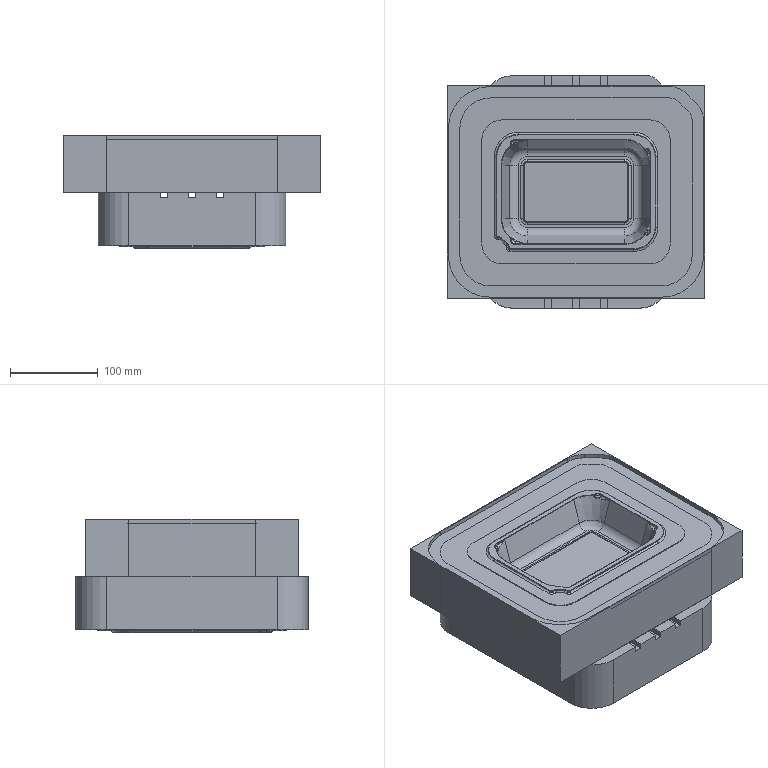NC program | NX | posted with a generic post | part box 293.342 x 265.342 x 129.5 mm
Lines 5002 to 6050 of 68427:
(B2 , TOOL : D8)
N10002 M6
N10004 G53
N10006 G17 G0 G90 X-89.051 Y-62.969 S7000 M3 M8
N10008 G43 Z215.5 H0
N10010 Z64.916
N10012 G94 G1 Z63.916 F4500.
N10014 X-86.104 Y-60.021
N10016 G3 X-86.104 Y-57.758 R1.6
N10018 G1 X-88.036 Y-55.826
N10020 G3 X-88.557 Y-55.61 R0.738
N10022 G1 X-89.227
N10024 G2 X-91.115 Y-55.286 R5.85
N10026 G3 X-93.151 Y-56.272 R1.6
N10028 G1 X-94.414 Y-59.905
N10030 Z64.916
N10032 G0 Z68.5
N10034 X-88.832 Y-63.392
N10036 Z64.582
N10038 G1 Z63.582
N10040 X-85.884 Y-60.444
N10042 G3 X-85.884 Y-58.182 R1.6
N10044 G1 X-88.119 Y-55.947
N10046 G3 X-88.585 Y-55.755 R0.659
N10048 G1 X-89.29
N10050 G2 X-91.54 Y-55.316 R5.876
N10052 G3 X-93.628 Y-56.189 R1.6
N10054 G1 X-95.087 Y-59.749
N10056 Z64.582
N10058 G0 Z68.5
N10060 X-85.268 Y-69.101
N10062 Z64.916
N10064 G1 Z63.916
N10066 X-81.645 Y-67.81
N10068 G3 X-80.676 Y-65.765 R1.6
N10070 G2 X-81.012 Y-63.966 R5.823
N10072 G1 X-81.021 Y-63.576
N10074 Y-63.147
N10076 G3 X-81.237 Y-62.625 R0.738
N10078 G1 X-83.165 Y-60.697
N10080 G3 X-85.428 Y-60.697 R1.6
N10082 G1 X-88.376 Y-63.645
N10084 Z64.916
N10086 G0 Z68.5
N10088 X-85.235 Y-69.546
N10090 Z64.582
N10092 G1 Z63.582
N10094 X-81.657 Y-68.134
N10096 G3 X-80.755 Y-66.059 R1.6
N10098 G2 X-81.165 Y-63.88 R5.875
N10100 G1 Y-63.173
N10102 G3 X-81.358 Y-62.708 R0.657
N10104 G1 X-83.586 Y-60.48
N10106 G3 X-85.849 Y-60.48 R1.6
N10108 G1 X-88.797 Y-63.428
N10110 Z64.582
N10112 G0 Z67.25
N10114 X-3.207 Y-76.775
N10116 Z64.248
N10118 G1 Z63.248
N10120 Y-71.505
N10122 G3 X-4.807 Y-69.905 R1.6
N10124 G1 X-75.383
N10126 G2 X-79.615 Y-68.143 R5.962
N10128 X-81.293 Y-63.949 R5.976
N10130 G1 Y-63.204
N10132 G3 X-81.468 Y-62.778 R0.602
N10134 G1 X-88.16 Y-56.086
N10136 G3 X-88.615 Y-55.882 R0.651
N10138 G1 X-89.43
N10140 G2 X-95.315 Y-49.996 R5.886
N10142 G1 Y40.358
N10144 G2 X-65.769 Y69.905 R29.546
N10146 G1 X65.769
N10148 G2 X95.315 Y40.358 R29.546
N10150 G1 Y-40.358
N10152 G2 X65.769 Y-69.905 R29.546
N10154 G1 X-4.807
N10156 G3 X-6.407 Y-71.505 R1.6
N10158 G1 Y-76.775
N10160 Z64.248
N10162 G0 Z66.582
N10164 X-3.207 Y-76.932
N10166 Z63.914
N10168 G1 Z62.914
N10170 Y-71.689
N10172 G3 X-4.807 Y-70.089 R1.6
N10174 G1 X-75.337
N10176 G2 X-81.476 Y-63.949 R6.037
N10178 G1 Y-63.242
N10180 G3 X-81.598 Y-62.908 R0.465
N10182 G1 X-88.314 Y-56.192
N10184 X-88.615 Y-56.066
N10186 X-89.359
N10188 G2 X-95.499 Y-49.926 R6.031
N10190 G1 Y40.358
N10192 G2 X-65.769 Y70.089 R29.73
N10194 G1 X65.769
N10196 G2 X95.499 Y40.358 R29.73
N10198 G1 Y-40.358
N10200 G2 X65.769 Y-70.089 R29.73
N10202 G1 X-4.807
N10204 G3 X-6.407 Y-71.689 R1.6
N10206 G1 Y-76.932
N10208 Z63.914
N10210 G0 Z67.25
N10212 X-89.345 Y-63.704
N10214 Z63.58
N10216 G1 Z62.58
N10218 X-86.397 Y-60.756
N10220 G3 X-86.397 Y-58.494 R1.6
N10222 G1 X-88.553 Y-56.338
N10224 X-89.359
N10226 G2 X-91.454 Y-56.019 R6.301
N10228 G3 X-93.476 Y-57.034 R1.6
N10230 G1 X-94.693 Y-60.705
N10232 Z63.58
N10234 G0 Z65.914
N10236 X-89.681 Y-63.963
N10238 Z63.246
N10240 G1 Z62.246
N10242 X-86.733 Y-61.015
N10244 G3 X-86.733 Y-58.753 R1.6
N10246 G1 X-88.727 Y-56.758
N10248 X-89.359
N10250 G2 X-91.462 Y-56.462 R6.706
N10252 G3 X-93.462 Y-57.52 R1.6
N10254 G1 X-94.606 Y-61.233
N10256 Z63.246
N10258 G0 Z65.58
N10260 X-90.266 Y-65.371
N10262 Z62.912
N10264 G1 Z61.912
N10266 X-87.026 Y-62.131
N10268 G3 X-87.026 Y-59.868 R1.6
N10270 G1 X-89.14 Y-57.754
N10272 X-89.359
N10274 X-89.736 Y-57.835
N10276 G2 X-91.734 Y-57.498 R8.299
N10278 G3 X-93.725 Y-58.574 R1.6
N10280 G1 X-94.849 Y-62.347
N10282 Z62.912
N10284 G0 Z65.914
N10286 X-86.139 Y-69.234
N10288 Z63.58
N10290 G1 Z62.58
N10292 X-82.463 Y-68.034
N10294 G3 X-81.438 Y-66.016 R1.6
N10296 G2 X-81.749 Y-63.949 R6.302
N10298 G1 Y-63.201
N10300 X-81.886 Y-63.005
N10302 X-83.898 Y-60.993
N10304 G3 X-86.161 Y-60.993 R1.6
N10306 G1 X-89.109 Y-63.941
N10308 Z63.58
N10310 G0 Z65.914
N10312 X-86.659 Y-69.16
N10314 Z63.246
N10316 G1 Z62.246
N10318 X-82.943 Y-68.027
N10320 G3 X-81.879 Y-66.031 R1.6
N10322 G2 X-82.169 Y-63.949 R6.707
N10324 G1 Y-63.316
N10326 X-84.157 Y-61.328
N10328 G3 X-86.42 Y-61.328 R1.6
N10330 G1 X-89.368 Y-64.276
N10332 Z63.246
N10334 G0 Z65.58
N10336 X-87.614 Y-69.717
N10338 Z62.912
N10340 G1 Z61.912
N10342 X-83.89 Y-68.513
N10344 G3 X-82.86 Y-66.499 R1.6
N10346 G2 X-83.136 Y-65.35 R7.681
N10348 G1 X-83.227 Y-64.658
N10350 X-83.165 Y-63.949
N10352 Y-63.729
N10354 X-85.305 Y-61.589
N10356 G3 X-87.568 Y-61.589 R1.6
N10358 G1 X-90.808 Y-64.828
N10360 Z62.912
N10362 G0 Z68.5
N10364 X-66.93 Y-46.786
N10366 Z64.916
N10368 G1 Z63.916
N10370 X-70.311 Y-48.522
N10372 G3 X-71.004 Y-50.676 R1.6
N10374 G2 X-70.442 Y-52.922 R5.1
N10376 G1 Y-54.729
N10378 G3 X-69.808 Y-55.362 R0.633
N10380 G1 X-65.313
N10382 G3 X-63.713 Y-53.762 R1.6
N10384 G1 Y-49.593
N10386 Z64.916
N10388 G0 Z68.5
N10390 X-67.282 Y-46.097
N10392 Z64.582
N10394 G1 Z63.582
N10396 X-70.524 Y-48.081
N10398 G3 X-71.054 Y-50.28 R1.6
N10400 G2 X-70.304 Y-52.9 R5.102
N10402 G1 Y-54.544
N10404 G3 X-69.617 Y-55.224 R0.637
N10406 G1 X-64.814
N10408 G3 X-63.214 Y-53.624 R1.6
N10410 G1 Y-49.455
N10412 Z64.582
N10414 G0 Z66.916
N10416 X-67.155 Y-46.069
N10418 Z64.248
N10420 G1 Z63.248
N10422 X-70.394 Y-48.045
N10424 G3 X-70.927 Y-50.244 R1.6
N10426 G2 X-70.195 Y-52.85 R5.005
N10428 G1 Y-54.428
N10430 G3 X-69.511 Y-55.116 R0.644
N10432 G1 X-64.717
N10434 G3 X-63.117 Y-53.516 R1.6
N10436 G1 Y-49.347
N10438 Z64.248
N10440 G0 Z66.582
N10442 X-67.095 Y-45.962
N10444 Z63.914
N10446 G1 Z62.914
N10448 X-70.321 Y-47.96
N10450 G3 X-70.838 Y-50.163 R1.6
N10452 G2 X-70.087 Y-52.8 R5.005
N10454 G1 Y-54.315
N10456 G3 X-69.399 Y-55.007 R0.645
N10458 G1 X-64.62
N10460 G3 X-63.02 Y-53.407 R1.6
N10462 G1 Y-49.238
N10464 Z63.914
N10466 G0 Z66.248
N10468 X-69.492 Y-43.606
N10470 Z63.58
N10472 G1 Z62.58
N10474 X-72.057 Y-46.534
N10476 G3 X-71.908 Y-48.792 R1.6
N10478 X-71.712 Y-48.962 R24.638
N10480 G2 X-69.978 Y-52.758 R4.995
N10482 G1 Y-54.08
N10484 G3 X-69.917 Y-54.513 R1.113
N10486 X-69.374 Y-54.898 R0.576
N10488 G1 X-55.815
N10490 X-55.672 Y-54.899
N10492 X-54.63
N10494 G3 X-53.03 Y-53.299 R1.6
N10496 G1 Y-49.129
N10498 Z63.58
N10500 G0 Z65.914
N10502 X-69.673 Y-42.848
N10504 Z63.246
N10506 G1 Z62.246
N10508 X-72.526 Y-45.89
N10510 G3 X-72.454 Y-48.151 R1.6
N10512 X-71.529 Y-48.976 R24.529
N10514 G2 X-69.832 Y-52.758 R4.93
N10516 G1 Y-53.896
N10518 X-69.768 Y-54.483
N10520 G3 X-69.314 Y-54.753 R0.536
N10522 G1 X-57.028
N10524 G3 X-55.672 Y-54.79 R24.529
N10526 G1 X-55.334
N10528 G3 X-53.734 Y-53.19 R1.6
N10530 G1 Y-48.984
N10532 Z63.246
N10534 G0 Z65.58
N10536 X-69.614 Y-42.69
N10538 Z62.912
N10540 G1 Z61.912
N10542 X-72.507 Y-45.754
N10544 G3 X-72.443 Y-48.015 R1.6
N10546 X-71.323 Y-49.01 R24.423
N10548 G2 X-69.625 Y-52.758 R4.854
N10550 G1 Y-54.235
N10552 G3 X-69.314 Y-54.546 R0.311
N10554 G1 X-58.27
N10556 G3 X-56.425 Y-54.673 R24.423
N10558 X-54.776 Y-53.123 R1.6
N10560 G1 X-54.645 Y-48.89
N10562 Z62.912
N10564 G0 Z65.246
N10566 X-66.724 Y-45.618
N10568 Z62.592
N10570 G1 Z61.592
N10572 X-69.8 Y-47.794
N10574 G3 X-70.182 Y-50.024 R1.6
N10576 G2 X-69.328 Y-52.711 R4.652
N10578 G1 Y-54.235
N10580 X-69.232 Y-54.248
N10582 X-64.5
N10584 G3 X-62.9 Y-52.648 R1.6
N10586 G1 Y-48.48
N10588 Z62.592
N10590 G0 Z64.912
N10592 X-66.784 Y-45.346
N10594 Z62.271
N10596 G1 Z61.271
N10598 X-69.734 Y-47.722
N10600 G3 X-69.976 Y-49.972 R1.6
N10602 G2 X-68.89 Y-52.941 R4.914
N10604 G1 Y-53.81
N10606 X-64.25
N10608 G3 X-62.65 Y-52.21 R1.6
N10610 G1 Y-48.041
N10612 Z62.271
N10614 G0 Z64.592
N10616 X-68.403 Y-43.794
N10618 Z61.951
N10620 G1 Z60.951
N10622 X-70.883 Y-46.932
N10624 G3 X-70.62 Y-49.179 R1.6
N10626 X-70.395 Y-49.354 R24.111
N10628 G2 X-68.028 Y-52.783 R6.451
N10630 G1 X-68.027 Y-52.798
N10632 X-68.013 Y-52.795
N10634 X-66.143
N10636 X-66.157 Y-52.699
N10638 X-66.066
N10640 G2 X-64.16 Y-53.051 R56.561
N10642 G3 X-64.168 Y-52.478 R2.
N10644 X-65.979 Y-51.121 R1.6
N10646 G1 X-63.674 Y-46.427
N10648 Z61.951
N10650 G0 Z68.5
N10652 X-63.691 Y49.593
N10654 Z64.916
N10656 G1 Z63.916
N10658 Y53.762
N10660 G3 X-65.291 Y55.362 R1.6
N10662 G1 X-69.794
N10664 G3 X-70.442 Y54.715 R0.648
N10666 G1 Y52.922
N10668 G2 X-71.009 Y50.666 R5.1
N10670 G3 X-70.321 Y48.51 R1.6
N10672 G1 X-66.944 Y46.767
N10674 Z64.916
N10676 G0 Z68.5
N10678 X-63.214 Y49.455
N10680 Z64.582
N10682 G1 Z63.582
N10684 Y53.624
N10686 G3 X-64.814 Y55.224 R1.6
N10688 G1 X-69.614
N10690 G3 X-70.304 Y54.544 R0.638
N10692 G1 Y52.9
N10694 G2 X-71.056 Y50.277 R5.106
N10696 G3 X-70.528 Y48.077 R1.6
N10698 G1 X-67.287 Y46.091
N10700 Z64.582
N10702 G0 Z66.916
N10704 X-63.116 Y49.347
N10706 Z64.248
N10708 G1 Z63.248
N10710 Y53.516
N10712 G3 X-64.716 Y55.116 R1.6
N10714 G1 X-69.51
N10716 G3 X-70.195 Y54.427 R0.644
N10718 G1 Y52.85
N10720 G2 X-70.933 Y50.235 R5.005
N10722 G3 X-70.405 Y48.034 R1.6
N10724 G1 X-67.169 Y46.052
N10726 Z64.248
N10728 G0 Z66.582
N10730 X-63.018 Y49.238
N10732 Z63.914
N10734 G1 Z62.914
N10736 Y53.407
N10738 G3 X-64.618 Y55.007 R1.6
N10740 G1 X-69.406
N10742 G3 X-70.087 Y54.314 R0.644
N10744 G1 Y52.8
N10746 G2 X-70.849 Y50.144 R5.005
N10748 G3 X-70.342 Y47.939 R1.6
N10750 G1 X-67.126 Y45.926
N10752 Z63.914
N10754 G0 Z66.248
N10756 X-53.149 Y49.129
N10758 Z63.58
N10760 G1 Z62.58
N10762 Y53.299
N10764 G3 X-54.749 Y54.899 R1.6
N10766 G1 X-55.672
N10768 G3 X-55.877 Y54.898 R24.638
N10770 G1 X-69.314
N10772 G3 X-69.914 Y54.541 R0.627
N10774 X-69.978 Y54.26 R0.655
N10776 G1 Y52.873
N10778 G2 X-71.712 Y48.962 R4.989
N10780 G1 X-71.801 Y48.886
N10782 G3 X-71.963 Y46.629 R1.6
N10784 G1 X-69.45 Y43.727
N10786 Z63.58
N10788 G0 Z65.914
N10790 X-53.714 Y48.984
N10792 Z63.246
N10794 G1 Z62.246
N10796 Y53.19
N10798 G3 X-55.314 Y54.79 R1.6
N10800 G1 X-55.672
N10802 G3 X-57.028 Y54.753 R24.529
N10804 G1 X-69.314
N10806 G3 X-69.77 Y54.477 R0.532
N10808 G1 X-69.832 Y53.896
N10810 Y52.758
N10812 G2 X-71.529 Y48.976 R4.93
N10814 G3 X-72.464 Y48.141 R24.529
N10816 X-72.535 Y45.879 R1.6
N10818 G1 X-69.678 Y42.837
N10820 Z63.246
N10822 G0 Z65.58
N10824 X-54.645 Y48.89
N10826 Z62.912
N10828 G1 Z61.912
N10830 X-54.776 Y53.123
N10832 G3 X-56.425 Y54.673 R1.6
N10834 X-58.27 Y54.546 R24.423
N10836 G1 X-69.314
N10838 G3 X-69.625 Y54.235 R0.311
N10840 G1 Y52.627
N10842 G2 X-71.315 Y49.017 R4.701
N10844 G3 X-72.291 Y48.158 R24.423
N10846 X-72.374 Y45.897 R1.6
N10848 G1 X-69.524 Y42.828
N10850 Z62.912
N10852 G0 Z65.246
N10854 X-62.901 Y48.48
N10856 Z62.592
N10858 G1 Z61.592
N10860 Y52.648
N10862 G3 X-64.501 Y54.248 R1.6
N10864 G1 X-69.328
N10866 Y52.792
N10868 G2 X-70.173 Y50.035 R4.642
N10870 G3 X-69.785 Y47.805 R1.6
N10872 G1 X-66.704 Y45.638
N10874 Z62.592
N10876 G0 Z64.912
N10878 X-62.623 Y48.041
N10880 Z62.271
N10882 G1 Z61.271
N10884 Y52.21
N10886 G3 X-64.223 Y53.81 R1.6
N10888 G1 X-68.89
N10890 Y52.941
N10892 G2 X-70.051 Y49.875 R4.855
N10894 G3 X-69.873 Y47.619 R1.6
N10896 G1 X-66.995 Y45.163
N10898 Z62.271
N10900 G0 Z64.592
N10902 X-63.694 Y46.406
N10904 Z61.951
N10906 G1 Z60.951
N10908 X-65.981 Y51.107
N10910 G3 X-64.17 Y52.463 R1.6
N10912 G1 X-64.164 Y52.511
N10914 G3 X-64.162 Y53.07 R2.
N10916 G1 X-64.384 Y53.021
N10918 X-64.904 Y52.902
N10920 X-65.023 Y52.844
N10922 G2 X-66.066 Y52.699 R6.755
N10924 G1 X-66.157
N10926 X-66.143 Y52.795
N10928 X-67.846
N10930 X-68.017 Y52.869
N10932 G2 X-70.395 Y49.354 R6.386
N10934 G3 X-70.626 Y49.174 R24.111
N10936 X-70.889 Y46.926 R1.6
N10938 G1 X-68.408 Y43.788
N10940 Z61.951
N10942 G0 Z64.271
N10944 X-1.6 Y-36.055
N10946 Z31.906
N10948 G1 Z30.906
N10950 Y-41.259
N10952 G3 X0. Y-42.859 R1.6
N10954 G1 X-55.672
N10956 G2 X-68.27 Y-30.261 R12.598
N10958 G1 Y30.261
N10960 G2 X-55.672 Y42.859 R12.598
N10962 G1 X55.672
N10964 G2 X68.27 Y30.261 R12.598
N10966 G1 Y-30.261
N10968 G2 X55.672 Y-42.859 R12.598
N10970 G1 X0.
N10972 G3 X1.6 Y-41.259 R1.6
N10974 G1 Y-36.055
N10976 Z31.906
N10978 G0 Z34.255
N10980 X-1.6 Y-35.567
N10982 Z31.558
N10984 G1 Z30.558
N10986 Y-40.795
N10988 G3 X0. Y-42.395 R1.6
N10990 G1 X-55.672
N10992 G2 X-67.806 Y-30.261 R12.134
N10994 G1 Y30.261
N10996 G2 X-55.672 Y42.395 R12.134
N10998 G1 X55.672
N11000 G2 X67.806 Y30.261 R12.134
N11002 G1 Y-30.261
N11004 G2 X55.672 Y-42.395 R12.134
N11006 G1 X0.
N11008 G3 X1.6 Y-40.795 R1.6
N11010 G1 Y-35.567
N11012 Z31.558
N11014 G0 Z33.906
N11016 X-1.6 Y-34.906
N11018 Z31.209
N11020 G1 Z30.209
N11022 Y-40.279
N11024 G3 X0. Y-41.879 R1.6
N11026 G1 X-55.672
N11028 G2 X-67.29 Y-30.261 R11.618
N11030 G1 Y30.261
N11032 G2 X-55.672 Y41.879 R11.618
N11034 G1 X55.672
N11036 G2 X67.29 Y30.261 R11.618
N11038 G1 Y-30.261
N11040 G2 X55.672 Y-41.879 R11.618
N11042 G1 X0.
N11044 G3 X1.6 Y-40.279 R1.6
N11046 G1 Y-34.906
N11048 Z31.209
N11050 G0 Z33.558
N11052 X24.785 Y-41.348
N11054 Z31.209
N11056 G1 X0. Z29.91
N11058 X-55.672
N11060 G2 X-66.759 Y-30.261 R11.087
N11062 G1 Y30.261
N11064 G2 X-55.672 Y41.348 R11.087
N11066 G1 X55.672
N11068 G2 X66.759 Y30.261 R11.087
N11070 G1 Y-30.261
N11072 G2 X55.672 Y-41.348 R11.087
N11074 G1 X0.
N11076 Y-38.656
N11078 X-55.672
N11080 G2 X-64.067 Y-30.261 R8.395
N11082 G1 Y30.261
N11084 G2 X-55.672 Y38.656 R8.395
N11086 G1 X55.672
N11088 G2 X64.067 Y30.261 R8.395
N11090 G1 Y-30.261
N11092 G2 X55.672 Y-38.656 R8.395
N11094 G1 X0.
N11096 G3 X-1.6 Y-40.256 R1.6
N11098 G1 Z30.91
N11100 G0 Z33.209
N11102 X24.785 Y-40.743
N11104 Z30.91
N11106 G1 X0. Z29.611
N11108 X-55.672
N11110 G2 X-66.154 Y-30.261 R10.482
N11112 G1 Y30.261
N11114 G2 X-55.672 Y40.743 R10.482
N11116 G1 X55.672
N11118 G2 X66.154 Y30.261 R10.482
N11120 G1 Y-30.261
N11122 G2 X55.672 Y-40.743 R10.482
N11124 G1 X0.
N11126 Y-39.051
N11128 X-55.672
N11130 G2 X-64.461 Y-30.261 R8.79
N11132 G1 Y30.261
N11134 G2 X-55.672 Y39.051 R8.79
N11136 G1 X55.672
N11138 G2 X64.461 Y30.261 R8.79
N11140 G1 Y-30.261
N11142 G2 X55.672 Y-39.051 R8.79
N11144 G1 X0.
N11146 G3 X-1.6 Y-40.651 R1.6
N11148 G1 Z30.611
N11150 G0 Z32.91
N11152 X24.785 Y-40.008
N11154 Z30.611
N11156 G1 X0. Z29.312
N11158 X-55.672
N11160 G2 X-65.419 Y-30.261 R9.747
N11162 G1 Y30.261
N11164 G2 X-55.672 Y40.008 R9.747
N11166 G1 X55.672
N11168 G2 X65.419 Y30.261 R9.747
N11170 G1 Y-30.261
N11172 G2 X55.672 Y-40.008 R9.747
N11174 G1 X0.
N11176 Y-39.462
N11178 X-55.672
N11180 G2 X-64.873 Y-30.261 R9.201
N11182 G1 Y30.261
N11184 G2 X-55.672 Y39.462 R9.201
N11186 G1 X55.672
N11188 G2 X64.873 Y30.261 R9.201
N11190 G1 Y-30.261
N11192 G2 X55.672 Y-39.462 R9.201
N11194 G1 X0.
N11196 G3 X-0.566 Y-39.696 R0.8
N11198 G1 Z30.312
N11200 G0 Z67.25
N11202 X1.6 Y-93.413
N11204 Z62.592
N11206 G1 Z61.592
N11208 Y-88.11
N11210 G3 X0. Y-86.51 R1.6
N11212 G1 X-83.671
N11214 G2 X-111.921 Y-58.26 R28.25
N11216 G1 Y58.26
N11218 G2 X-83.671 Y86.51 R28.25
N11220 G1 X83.671
N11222 G2 X111.921 Y58.26 R28.25
N11224 G1 Y-58.26
N11226 G2 X83.671 Y-86.51 R28.25
N11228 G1 X0.
N11230 G3 X-1.6 Y-88.11 R1.6
N11232 G1 Y-93.413
N11234 Z62.592
N11236 G0 Z64.912
N11238 X1.6 Y-93.541
N11240 Z62.271
N11242 G1 Z61.271
N11244 Y-88.11
N11246 G3 X0. Y-86.51 R1.6
N11248 G1 X-83.671
N11250 G2 X-111.921 Y-58.26 R28.25
N11252 G1 Y58.26
N11254 G2 X-83.671 Y86.51 R28.25
N11256 G1 X83.671
N11258 G2 X111.921 Y58.26 R28.25
N11260 G1 Y-58.26
N11262 G2 X83.671 Y-86.51 R28.25
N11264 G1 X0.
N11266 G3 X-1.6 Y-88.11 R1.6
N11268 G1 Y-93.541
N11270 Z62.271
N11272 G0 Z64.592
N11274 X1.6 Y-94.046
N11276 Z61.951
N11278 G1 Z60.951
N11280 Y-88.11
N11282 G3 X0. Y-86.51 R1.6
N11284 G1 X-83.671
N11286 G2 X-111.921 Y-58.26 R28.25
N11288 G1 Y58.26
N11290 G2 X-83.671 Y86.51 R28.25
N11292 G1 X83.671
N11294 G2 X111.921 Y58.26 R28.25
N11296 G1 Y-58.26
N11298 G2 X83.671 Y-86.51 R28.25
N11300 G1 X0.
N11302 G3 X-1.6 Y-88.11 R1.6
N11304 G1 Y-94.046
N11306 Z61.951
N11308 G0 Z64.271
N11310 X1.6 Y-94.049
N11312 Z61.912
N11314 G1 Z60.912
N11316 Y-88.11
N11318 G3 X0. Y-86.51 R1.6
N11320 G1 X-83.671
N11322 G2 X-111.921 Y-58.26 R28.25
N11324 G1 Y58.26
N11326 G2 X-83.671 Y86.51 R28.25
N11328 G1 X83.671
N11330 G2 X111.921 Y58.26 R28.25
N11332 G1 Y-58.26
N11334 G2 X83.671 Y-86.51 R28.25
N11336 G1 X0.
N11338 G3 X-1.6 Y-88.11 R1.6
N11340 G1 Y-94.049
N11342 Z61.912
N11344 G0 Z67.25
N11346 X5.993 Y108.93
N11348 Z62.592
N11350 G1 Z61.592
N11352 Y114.41
N11354 G3 X4.393 Y116.01 R1.6
N11356 G1 X106.458
N11358 G2 X123.252 Y109.054 R23.75
N11360 G1 X134.465 Y97.841
N11362 G2 X141.421 Y81.047 R23.75
N11364 G1 Y-72.26
N11366 G2 X97.671 Y-116.01 R43.75
N11368 G1 X-97.671
N11370 G2 X-141.421 Y-72.26 R43.75
N11372 G1 Y72.26
N11374 G2 X-97.671 Y116.01 R43.75
N11376 G1 X4.393
N11378 G3 X2.793 Y114.41 R1.6
N11380 G1 Y108.93
N11382 Z62.592
N11384 G0 Z64.912
N11386 X5.993 Y108.949
N11388 Z62.271
N11390 G1 Z61.271
N11392 Y114.41
N11394 G3 X4.393 Y116.01 R1.6
N11396 G1 X106.458
N11398 G2 X123.252 Y109.054 R23.75
N11400 G1 X134.465 Y97.841
N11402 G2 X141.421 Y81.047 R23.75
N11404 G1 Y-72.26
N11406 G2 X97.671 Y-116.01 R43.75
N11408 G1 X-97.671
N11410 G2 X-141.421 Y-72.26 R43.75
N11412 G1 Y72.26
N11414 G2 X-97.671 Y116.01 R43.75
N11416 G1 X4.393
N11418 G3 X2.793 Y114.41 R1.6
N11420 G1 Y108.949
N11422 Z62.271
N11424 G0 Z64.592
N11426 X5.993 Y108.47
N11428 Z61.951
N11430 G1 Z60.951
N11432 Y114.41
N11434 G3 X4.393 Y116.01 R1.6
N11436 G1 X106.458
N11438 G2 X123.252 Y109.054 R23.75
N11440 G1 X134.465 Y97.841
N11442 G2 X141.421 Y81.047 R23.75
N11444 G1 Y-72.26
N11446 G2 X97.671 Y-116.01 R43.75
N11448 G1 X-97.671
N11450 G2 X-141.421 Y-72.26 R43.75
N11452 G1 Y72.26
N11454 G2 X-97.671 Y116.01 R43.75
N11456 G1 X4.393
N11458 G3 X2.793 Y114.41 R1.6
N11460 G1 Y108.47
N11462 Z61.951
N11464 G0 Z64.271
N11466 X5.993
N11468 Z61.912
N11470 G1 Z60.912
N11472 Y114.41
N11474 G3 X4.393 Y116.01 R1.6
N11476 G1 X106.458
N11478 G2 X123.252 Y109.054 R23.75
N11480 G1 X134.465 Y97.841
N11482 G2 X141.421 Y81.047 R23.75
N11484 G1 Y-72.26
N11486 G2 X97.671 Y-116.01 R43.75
N11488 G1 X-97.671
N11490 G2 X-141.421 Y-72.26 R43.75
N11492 G1 Y72.26
N11494 G2 X-97.671 Y116.01 R43.75
N11496 G1 X4.393
N11498 G3 X2.793 Y114.41 R1.6
N11500 G1 Y108.47
N11502 Z61.912
N11504 G0 Z68.5
N11506 X75.004 Y38.28
N11508 Z64.916
N11510 G1 Z63.916
N11512 X79.173
N11514 G3 X80.773 Y39.88 R1.6
N11516 G1 Y44.379
N11518 G3 X80.121 Y45.031 R0.652
N11520 G1 X78.333
N11522 G2 X76.097 Y45.569 R4.916
N11524 G3 X73.944 Y44.871 R1.6
N11526 G1 X72.221 Y41.498
N11528 Z64.916
N11530 G0 Z68.5
N11532 X74.866 Y37.803
N11534 Z64.582
N11536 G1 Z63.582
N11538 X79.035
N11540 G3 X80.635 Y39.403 R1.6
N11542 G1 Y44.199
N11544 G3 X79.955 Y44.893 R0.638
N11546 G1 X78.31
N11548 G2 X76.619 Y45.195 R5.532
N11550 X75.636 Y45.665 R4.815
N11552 G3 X73.431 Y45.157 R1.6
N11554 G1 X71.42 Y41.944
N11556 Z64.582
N11558 G0 Z66.916
N11560 X74.758 Y37.706
N11562 Z64.248
N11564 G1 Z63.248
N11566 X78.927
N11568 G3 X80.527 Y39.306 R1.6
N11570 G1 Y44.09
N11572 G3 X79.846 Y44.785 R0.647
N11574 G1 X78.261
N11576 G2 X75.651 Y45.519 R5.005
N11578 G3 X73.451 Y44.988 R1.6
N11580 G1 X71.473 Y41.75
N11582 Z64.248
N11584 G0 Z66.582
N11586 X74.649 Y37.605
N11588 Z63.914
N11590 G1 Z62.914
N11592 X78.818
N11594 G3 X80.418 Y39.205 R1.6
N11596 G1 Y43.982
N11598 G3 X79.726 Y44.676 R0.642
N11600 G1 X78.211
N11602 G2 X75.541 Y45.448 R5.005
N11604 G3 X73.334 Y44.947 R1.6
N11606 G1 X71.311 Y41.738
N11608 Z63.914
N11610 G0 Z66.248
N11612 X74.54 Y27.738
N11614 Z63.58
N11616 G1 Z62.58
N11618 X78.71
N11620 G3 X80.31 Y29.338 R1.6
N11622 G1 Y30.261
N11624 G3 X80.309 Y30.48 R24.638
N11626 G1 Y43.957
N11628 G3 X79.699 Y44.567 R0.61
N11630 G1 X78.169
N11632 G2 X74.373 Y46.301 R4.995
N11634 G1 X74.258 Y46.434
N11636 G3 X72.001 Y46.591 R1.6
N11638 G1 X69.089 Y44.057
N11640 Z63.58
N11642 G0 Z65.914
N11644 X74.394 Y28.323
N11646 Z63.246
N11648 G1 Z62.246
N11650 X78.601
N11652 G3 X80.201 Y29.923 R1.6
N11654 G1 Y30.261
N11656 G3 X80.164 Y31.617 R24.529
N11658 G1 Y43.904
N11660 G3 X79.645 Y44.422 R0.518
N11662 G1 X78.169
N11664 G2 X74.386 Y46.118 R4.93
N11666 G3 X73.438 Y47.173 R24.529
N11668 X71.176 Y47.229 R1.6
N11670 G1 X68.133 Y44.332
N11672 Z63.246
N11674 G0 Z65.58
N11676 X74.3 Y29.235
N11678 Z62.912
N11680 G1 Z61.912
N11682 X78.533 Y29.365
N11684 G3 X80.083 Y31.014 R1.6
N11686 X79.956 Y32.859 R24.423
N11688 G1 Y43.799
N11690 G3 X79.921 Y44.023 R0.725
N11692 X79.657 Y44.215 R0.277
N11694 G1 X78.169
N11696 G2 X74.421 Y45.912 R4.854
N11698 G3 X73.39 Y47.071 R24.423
N11700 X71.128 Y47.13 R1.6
N11702 G1 X68.066 Y44.225
N11704 Z62.912
N11706 G0 Z65.246
N11708 X73.89 Y37.49
N11710 Z62.592
N11712 G1 Z61.592
N11714 X78.059
N11716 G3 X79.659 Y39.09 R1.6
N11718 G1 Y43.917
N11720 X78.169
N11722 G2 X75.401 Y44.808 R4.764
N11724 G3 X73.169 Y44.439 R1.6
N11726 G1 X70.97 Y41.368
N11728 Z62.592
N11730 G0 Z64.912
N11732 X73.452 Y37.212
N11734 Z62.271
N11736 G1 Z61.271
N11738 X77.621
N11740 G3 X79.221 Y38.812 R1.6
N11742 G1 Y43.479
N11744 X78.353
N11746 G2 X75.286 Y44.64 R4.857
N11748 G3 X73.03 Y44.461 R1.6
N11750 G1 X70.575 Y41.583
N11752 Z62.271
N11754 G0 Z64.592
N11756 X73.268 Y35.944
N11758 Z61.951
N11760 G1 Z60.951
N11762 X77.246 Y36.787
N11764 G3 X78.48 Y38.683 R1.6
N11766 G2 X78.106 Y40.543 R92.711
N11768 G1 X78.084 Y40.614
N11770 X78.132 Y40.673
N11772 X78.206 Y40.667
N11774 Y42.544
N11776 X78.243 Y42.541
N11778 X78.259 Y42.579
N11780 X78.23 Y42.603
N11782 G2 X74.763 Y44.987 R6.398
N11784 G3 X74.607 Y45.186 R24.111
N11786 X72.36 Y45.453 R1.6
N11788 G1 X69.222 Y42.979
N11790 Z61.951
N11792 G0 Z68.5
N11794 X72.199 Y-41.518
N11796 Z64.916
N11798 G1 Z63.916
N11800 X73.933 Y-44.898
N11802 G3 X76.087 Y-45.591 R1.6
N11804 G2 X78.333 Y-45.031 R5.08
N11806 G1 X80.121
N11808 G3 X80.773 Y-44.379 R0.652
N11810 G1 Y-39.9
N11812 G3 X79.173 Y-38.3 R1.6
N11814 G1 X75.004
N11816 Z64.916
N11818 G0 Z68.5
N11820 X71.38 Y-41.986
N11822 Z64.582
N11824 G1 Z63.582
N11826 X73.41 Y-45.185
N11828 G3 X75.618 Y-45.679 R1.6
N11830 G2 X77.866 Y-44.928 R4.92
N11832 G1 X78.31 Y-44.893
N11834 X79.955
N11836 G3 X80.399 Y-44.772 R1.099
N11838 X80.635 Y-44.213 R0.747
N11840 G1 Y-39.403
N11842 G3 X79.035 Y-37.803 R1.6
N11844 G1 X74.866
N11846 Z64.582
N11848 G0 Z66.916
N11850 X71.481 Y-41.743
N11852 Z64.248
N11854 G1 Z63.248
N11856 X73.456 Y-44.983
N11858 G3 X75.655 Y-45.516 R1.6
N11860 G2 X78.261 Y-44.785 R5.005
N11862 G1 X79.846
N11864 G3 X80.527 Y-44.104 R0.644
N11866 G1 Y-39.306
N11868 G3 X78.927 Y-37.706 R1.6
N11870 G1 X74.758
N11872 Z64.248
N11874 G0 Z66.582
N11876 X71.375 Y-41.683
N11878 Z63.914
N11880 G1 Z62.914
N11882 X73.372 Y-44.909
N11884 G3 X75.575 Y-45.426 R1.6
N11886 G2 X78.211 Y-44.676 R5.005
N11888 G1 X79.737
N11890 G3 X80.418 Y-43.996 R0.641
N11892 G1 Y-39.209
N11894 G3 X78.818 Y-37.609 R1.6
N11896 G1 X74.649
N11898 Z63.914
N11900 G0 Z66.248
N11902 X69.015 Y-44.082
N11904 Z63.58
N11906 G1 Z62.58
N11908 X71.943 Y-46.648
N11910 G3 X74.201 Y-46.499 R1.6
N11912 X74.373 Y-46.301 R24.638
N11914 G2 X78.169 Y-44.567 R4.995
N11916 G1 X79.697
N11918 G3 X80.309 Y-43.955 R0.612
N11920 G1 Y-30.487
N11922 Y-30.396
N11924 X80.31 Y-30.261
N11926 Y-29.22
N11928 G3 X78.71 Y-27.62 R1.6
N11930 G1 X74.54
N11932 Z63.58
N11934 G0 Z65.914
N11936 X68.255 Y-44.264
N11938 Z63.246
N11940 G1 Z62.246
N11942 X71.297 Y-47.118
N11944 G3 X73.559 Y-47.046 R1.6
N11946 X74.386 Y-46.118 R24.529
N11948 G2 X78.169 Y-44.422 R4.93
N11950 G1 X79.645
N11952 G3 X80.164 Y-43.904 R0.518
N11954 G1 Y-31.617
N11956 G3 X80.201 Y-30.261 R24.529
N11958 G1 Y-29.923
N11960 G3 X78.601 Y-28.323 R1.6
N11962 G1 X74.394
N11964 Z63.246
N11966 G0 Z65.58
N11968 X68.102 Y-44.203
N11970 Z62.912
N11972 G1 Z61.912
N11974 X71.165 Y-47.096
N11976 G3 X73.427 Y-47.032 R1.6
N11978 X74.421 Y-45.912 R24.423
N11980 G2 X78.169 Y-44.215 R4.854
N11982 G1 X79.682
N11984 G3 X79.918 Y-44.034 R0.244
N11986 X79.956 Y-43.743 R1.119
N11988 G1 Y-32.859
N11990 G3 X80.083 Y-31.014 R24.423
N11992 X78.533 Y-29.365 R1.6
N11994 G1 X74.3 Y-29.235
N11996 Z62.912
N11998 G0 Z65.246
N12000 X70.961 Y-41.376
N12002 Z62.592
N12004 G1 Z61.592
N12006 X73.164 Y-44.444
N12008 G3 X75.396 Y-44.811 R1.6
N12010 G2 X78.169 Y-43.917 R4.764
N12012 G1 X79.649
N12014 X79.659 Y-43.732
N12016 Y-39.089
N12018 G3 X78.059 Y-37.489 R1.6
N12020 G1 X73.89
N12022 Z62.592
N12024 G0 Z64.912
N12026 X70.783 Y-41.348
N12028 Z62.271
N12030 G1 Z61.271
N12032 X73.15 Y-44.299
N12034 G3 X75.4 Y-44.547 R1.6
N12036 G2 X78.352 Y-43.479 R4.858
N12038 G1 X79.221
N12040 Y-38.839
N12042 G3 X77.621 Y-37.239 R1.6
N12044 G1 X73.452
N12046 Z62.271
N12048 G0 Z64.592
N12050 X69.217 Y-42.984
N12052 Z61.951
N12054 G1 Z60.951
N12056 X72.355 Y-45.459
N12058 G3 X74.602 Y-45.194 R1.6
N12060 X74.765 Y-44.984 R24.111
N12062 G2 X78.23 Y-42.618 R6.312
N12064 G1 X78.206 Y-42.559
N12066 Y-40.734
N12068 X78.146 Y-40.772
N12070 X78.082 Y-40.73
N12072 X78.094 Y-40.66
N12074 X78.221 Y-39.763
N12076 X78.455 Y-38.75
N12078 G3 X77.596 Y-38.829 R2.
N12080 X76.188 Y-40.486 R2.
N12082 X76.347 Y-41.077 R0.8
N12084 G1 X71.841 Y-38.261
N12086 Z61.951
N12088 G0 Z215.5
N12090 M9
N12092 M5